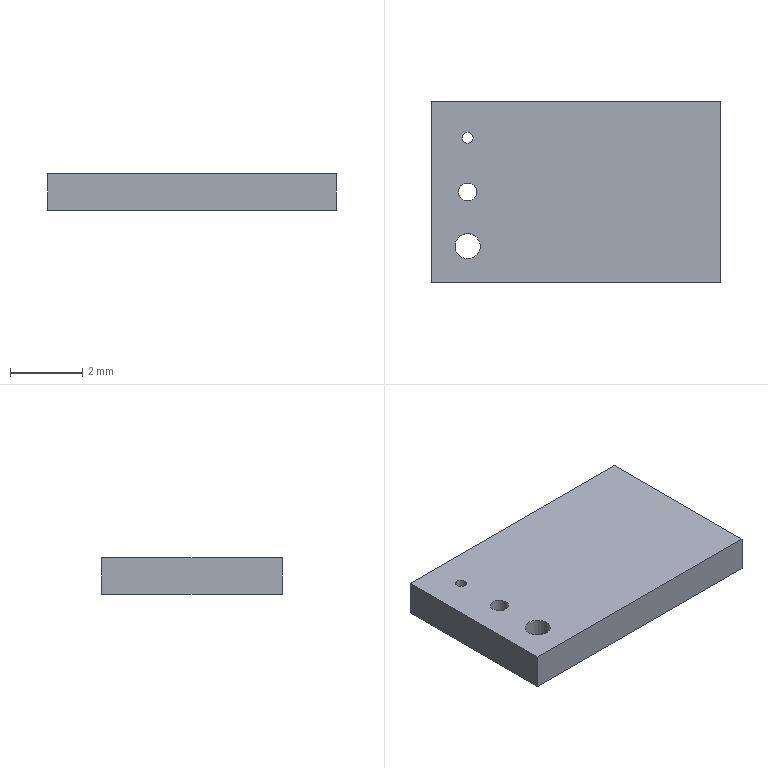Part | SolidWorks | features ICE 2, Extrusion 1 | 1 solid | 12 faces | box 8 x 5 x 1 mm | volume 39.348 mm3 | cylinder 6 | plane 6 | commonest cylinder face diameters 0.3 x2 0.5 x2 0.7 x2
STEP:
#1=CARTESIAN_POINT('',(0.85,-1.5,0.));
#2=VERTEX_POINT('',#1);
#3=CARTESIAN_POINT('',(1.15,-1.5,0.));
#4=VERTEX_POINT('',#3);
#5=CARTESIAN_POINT('',(1.,-1.5,0.));
#6=DIRECTION('',(0.,0.,1.));
#7=DIRECTION('',(1.,0.,0.));
#8=AXIS2_PLACEMENT_3D('',#5,#6,#7);
#9=CIRCLE('',#8,0.15);
#10=EDGE_CURVE('',#2,#4,#9,.T.);
#11=ORIENTED_EDGE('',*,*,#10,.F.);
#12=CARTESIAN_POINT('',(0.85,-1.5,1.));
#13=VERTEX_POINT('',#12);
#14=CARTESIAN_POINT('',(0.85,-1.5,-1.));
#15=DIRECTION('',(0.,0.,1.));
#16=VECTOR('',#15,1000.);
#17=LINE('',#14,#16);
#18=EDGE_CURVE('',#2,#13,#17,.T.);
#19=ORIENTED_EDGE('',*,*,#18,.T.);
#20=CARTESIAN_POINT('',(1.15,-1.5,1.));
#21=VERTEX_POINT('',#20);
#22=CARTESIAN_POINT('',(1.,-1.5,1.));
#23=DIRECTION('',(0.,0.,1.));
#24=DIRECTION('',(1.,0.,0.));
#25=AXIS2_PLACEMENT_3D('',#22,#23,#24);
#26=CIRCLE('',#25,0.15);
#27=EDGE_CURVE('',#13,#21,#26,.T.);
#28=ORIENTED_EDGE('',*,*,#27,.T.);
#29=CARTESIAN_POINT('',(1.15,-1.5,-1.));
#30=DIRECTION('',(0.,0.,1.));
#31=VECTOR('',#30,1000.);
#32=LINE('',#29,#31);
#33=EDGE_CURVE('',#4,#21,#32,.T.);
#34=ORIENTED_EDGE('',*,*,#33,.F.);
#35=EDGE_LOOP('',(#11,#19,#28,#34));
#36=FACE_OUTER_BOUND('',#35,.T.);
#37=CARTESIAN_POINT('',(1.,-1.5,-1.));
#38=DIRECTION('',(0.,0.,1.));
#39=DIRECTION('',(1.,0.,0.));
#40=AXIS2_PLACEMENT_3D('',#37,#38,#39);
#41=CYLINDRICAL_SURFACE('',#40,0.15);
#42=ADVANCED_FACE('',(#36),#41,.F.);
#43=CARTESIAN_POINT('',(0.75,-3.,0.));
#44=VERTEX_POINT('',#43);
#45=CARTESIAN_POINT('',(1.25,-3.,0.));
#46=VERTEX_POINT('',#45);
#47=CARTESIAN_POINT('',(1.,-3.,0.));
#48=DIRECTION('',(0.,0.,1.));
#49=DIRECTION('',(1.,0.,0.));
#50=AXIS2_PLACEMENT_3D('',#47,#48,#49);
#51=CIRCLE('',#50,0.25);
#52=EDGE_CURVE('',#44,#46,#51,.T.);
#53=ORIENTED_EDGE('',*,*,#52,.F.);
#54=CARTESIAN_POINT('',(0.75,-3.,1.));
#55=VERTEX_POINT('',#54);
#56=CARTESIAN_POINT('',(0.75,-3.,-1.));
#57=DIRECTION('',(0.,0.,1.));
#58=VECTOR('',#57,1000.);
#59=LINE('',#56,#58);
#60=EDGE_CURVE('',#44,#55,#59,.T.);
#61=ORIENTED_EDGE('',*,*,#60,.T.);
#62=CARTESIAN_POINT('',(1.25,-3.,1.));
#63=VERTEX_POINT('',#62);
#64=CARTESIAN_POINT('',(1.,-3.,1.));
#65=DIRECTION('',(0.,0.,1.));
#66=DIRECTION('',(1.,0.,0.));
#67=AXIS2_PLACEMENT_3D('',#64,#65,#66);
#68=CIRCLE('',#67,0.25);
#69=EDGE_CURVE('',#55,#63,#68,.T.);
#70=ORIENTED_EDGE('',*,*,#69,.T.);
#71=CARTESIAN_POINT('',(1.25,-3.,-1.));
#72=DIRECTION('',(0.,0.,1.));
#73=VECTOR('',#72,1000.);
#74=LINE('',#71,#73);
#75=EDGE_CURVE('',#46,#63,#74,.T.);
#76=ORIENTED_EDGE('',*,*,#75,.F.);
#77=EDGE_LOOP('',(#53,#61,#70,#76));
#78=FACE_OUTER_BOUND('',#77,.T.);
#79=CARTESIAN_POINT('',(1.,-3.,-1.));
#80=DIRECTION('',(0.,0.,1.));
#81=DIRECTION('',(1.,0.,0.));
#82=AXIS2_PLACEMENT_3D('',#79,#80,#81);
#83=CYLINDRICAL_SURFACE('',#82,0.25);
#84=ADVANCED_FACE('',(#78),#83,.F.);
#85=CARTESIAN_POINT('',(0.65,-4.5,0.));
#86=VERTEX_POINT('',#85);
#87=CARTESIAN_POINT('',(1.35,-4.5,0.));
#88=VERTEX_POINT('',#87);
#89=CARTESIAN_POINT('',(1.,-4.5,0.));
#90=DIRECTION('',(0.,0.,1.));
#91=DIRECTION('',(1.,0.,0.));
#92=AXIS2_PLACEMENT_3D('',#89,#90,#91);
#93=CIRCLE('',#92,0.35);
#94=EDGE_CURVE('',#86,#88,#93,.T.);
#95=ORIENTED_EDGE('',*,*,#94,.F.);
#96=CARTESIAN_POINT('',(0.65,-4.5,1.));
#97=VERTEX_POINT('',#96);
#98=CARTESIAN_POINT('',(0.65,-4.5,-1.));
#99=DIRECTION('',(0.,0.,1.));
#100=VECTOR('',#99,1000.);
#101=LINE('',#98,#100);
#102=EDGE_CURVE('',#86,#97,#101,.T.);
#103=ORIENTED_EDGE('',*,*,#102,.T.);
#104=CARTESIAN_POINT('',(1.35,-4.5,1.));
#105=VERTEX_POINT('',#104);
#106=CARTESIAN_POINT('',(1.,-4.5,1.));
#107=DIRECTION('',(0.,0.,1.));
#108=DIRECTION('',(1.,0.,0.));
#109=AXIS2_PLACEMENT_3D('',#106,#107,#108);
#110=CIRCLE('',#109,0.35);
#111=EDGE_CURVE('',#97,#105,#110,.T.);
#112=ORIENTED_EDGE('',*,*,#111,.T.);
#113=CARTESIAN_POINT('',(1.35,-4.5,-1.));
#114=DIRECTION('',(0.,0.,1.));
#115=VECTOR('',#114,1000.);
#116=LINE('',#113,#115);
#117=EDGE_CURVE('',#88,#105,#116,.T.);
#118=ORIENTED_EDGE('',*,*,#117,.F.);
#119=EDGE_LOOP('',(#95,#103,#112,#118));
#120=FACE_OUTER_BOUND('',#119,.T.);
#121=CARTESIAN_POINT('',(1.,-4.5,-1.));
#122=DIRECTION('',(0.,0.,1.));
#123=DIRECTION('',(1.,0.,0.));
#124=AXIS2_PLACEMENT_3D('',#121,#122,#123);
#125=CYLINDRICAL_SURFACE('',#124,0.35);
#126=ADVANCED_FACE('',(#120),#125,.F.);
#127=CARTESIAN_POINT('',(0.,-0.5,1.));
#128=VERTEX_POINT('',#127);
#129=CARTESIAN_POINT('',(0.,-5.5,1.));
#130=VERTEX_POINT('',#129);
#131=CARTESIAN_POINT('',(0.,0.,1.));
#132=DIRECTION('',(0.,-1.,0.));
#133=VECTOR('',#132,1000.);
#134=LINE('',#131,#133);
#135=EDGE_CURVE('',#128,#130,#134,.T.);
#136=ORIENTED_EDGE('',*,*,#135,.F.);
#137=CARTESIAN_POINT('',(0.,-0.5,0.));
#138=VERTEX_POINT('',#137);
#139=CARTESIAN_POINT('',(0.,-0.5,-6.));
#140=DIRECTION('',(0.,0.,1.));
#141=VECTOR('',#140,1000.);
#142=LINE('',#139,#141);
#143=EDGE_CURVE('',#138,#128,#142,.T.);
#144=ORIENTED_EDGE('',*,*,#143,.F.);
#145=CARTESIAN_POINT('',(0.,-5.5,0.));
#146=VERTEX_POINT('',#145);
#147=CARTESIAN_POINT('',(0.,0.,0.));
#148=DIRECTION('',(0.,-1.,0.));
#149=VECTOR('',#148,1000.);
#150=LINE('',#147,#149);
#151=EDGE_CURVE('',#138,#146,#150,.T.);
#152=ORIENTED_EDGE('',*,*,#151,.T.);
#153=CARTESIAN_POINT('',(0.,-5.5,-6.));
#154=DIRECTION('',(0.,0.,1.));
#155=VECTOR('',#154,1000.);
#156=LINE('',#153,#155);
#157=EDGE_CURVE('',#146,#130,#156,.T.);
#158=ORIENTED_EDGE('',*,*,#157,.T.);
#159=EDGE_LOOP('',(#136,#144,#152,#158));
#160=FACE_OUTER_BOUND('',#159,.T.);
#161=CARTESIAN_POINT('',(0.,0.,1.));
#162=DIRECTION('',(1.,0.,0.));
#163=DIRECTION('',(0.,1.,0.));
#164=AXIS2_PLACEMENT_3D('',#161,#162,#163);
#165=PLANE('',#164);
#166=ADVANCED_FACE('',(#160),#165,.F.);
#167=CARTESIAN_POINT('',(8.,-5.5,0.));
#168=VERTEX_POINT('',#167);
#169=CARTESIAN_POINT('',(8.,-0.5,0.));
#170=VERTEX_POINT('',#169);
#171=CARTESIAN_POINT('',(8.,0.,0.));
#172=DIRECTION('',(0.,1.,0.));
#173=VECTOR('',#172,1000.);
#174=LINE('',#171,#173);
#175=EDGE_CURVE('',#168,#170,#174,.T.);
#176=ORIENTED_EDGE('',*,*,#175,.T.);
#177=CARTESIAN_POINT('',(8.,-0.5,1.));
#178=VERTEX_POINT('',#177);
#179=CARTESIAN_POINT('',(8.,-0.5,-6.));
#180=DIRECTION('',(0.,0.,1.));
#181=VECTOR('',#180,1000.);
#182=LINE('',#179,#181);
#183=EDGE_CURVE('',#170,#178,#182,.T.);
#184=ORIENTED_EDGE('',*,*,#183,.T.);
#185=CARTESIAN_POINT('',(8.,-5.5,1.));
#186=VERTEX_POINT('',#185);
#187=CARTESIAN_POINT('',(8.,0.,1.));
#188=DIRECTION('',(0.,1.,0.));
#189=VECTOR('',#188,1000.);
#190=LINE('',#187,#189);
#191=EDGE_CURVE('',#186,#178,#190,.T.);
#192=ORIENTED_EDGE('',*,*,#191,.F.);
#193=CARTESIAN_POINT('',(8.,-5.5,-6.));
#194=DIRECTION('',(0.,0.,1.));
#195=VECTOR('',#194,1000.);
#196=LINE('',#193,#195);
#197=EDGE_CURVE('',#168,#186,#196,.T.);
#198=ORIENTED_EDGE('',*,*,#197,.F.);
#199=EDGE_LOOP('',(#176,#184,#192,#198));
#200=FACE_OUTER_BOUND('',#199,.T.);
#201=CARTESIAN_POINT('',(8.,0.,1.));
#202=DIRECTION('',(-1.,0.,0.));
#203=DIRECTION('',(0.,-1.,0.));
#204=AXIS2_PLACEMENT_3D('',#201,#202,#203);
#205=PLANE('',#204);
#206=ADVANCED_FACE('',(#200),#205,.F.);
#207=CARTESIAN_POINT('',(0.,-0.5,1.));
#208=DIRECTION('',(1.,0.,0.));
#209=VECTOR('',#208,1000.);
#210=LINE('',#207,#209);
#211=EDGE_CURVE('',#128,#178,#210,.T.);
#212=ORIENTED_EDGE('',*,*,#211,.F.);
#213=ORIENTED_EDGE('',*,*,#135,.T.);
#214=CARTESIAN_POINT('',(0.,-5.5,1.));
#215=DIRECTION('',(-1.,0.,0.));
#216=VECTOR('',#215,1000.);
#217=LINE('',#214,#216);
#218=EDGE_CURVE('',#186,#130,#217,.T.);
#219=ORIENTED_EDGE('',*,*,#218,.F.);
#220=ORIENTED_EDGE('',*,*,#191,.T.);
#221=EDGE_LOOP('',(#212,#213,#219,#220));
#222=FACE_OUTER_BOUND('',#221,.T.);
#223=CARTESIAN_POINT('',(1.,-1.5,1.));
#224=DIRECTION('',(0.,0.,1.));
#225=DIRECTION('',(1.,0.,0.));
#226=AXIS2_PLACEMENT_3D('',#223,#224,#225);
#227=CIRCLE('',#226,0.15);
#228=EDGE_CURVE('',#21,#13,#227,.T.);
#229=ORIENTED_EDGE('',*,*,#228,.F.);
#230=ORIENTED_EDGE('',*,*,#27,.F.);
#231=EDGE_LOOP('',(#229,#230));
#232=FACE_BOUND('',#231,.T.);
#233=CARTESIAN_POINT('',(1.,-3.,1.));
#234=DIRECTION('',(0.,0.,1.));
#235=DIRECTION('',(1.,0.,0.));
#236=AXIS2_PLACEMENT_3D('',#233,#234,#235);
#237=CIRCLE('',#236,0.25);
#238=EDGE_CURVE('',#63,#55,#237,.T.);
#239=ORIENTED_EDGE('',*,*,#238,.F.);
#240=ORIENTED_EDGE('',*,*,#69,.F.);
#241=EDGE_LOOP('',(#239,#240));
#242=FACE_BOUND('',#241,.T.);
#243=CARTESIAN_POINT('',(1.,-4.5,1.));
#244=DIRECTION('',(0.,0.,1.));
#245=DIRECTION('',(1.,0.,0.));
#246=AXIS2_PLACEMENT_3D('',#243,#244,#245);
#247=CIRCLE('',#246,0.35);
#248=EDGE_CURVE('',#105,#97,#247,.T.);
#249=ORIENTED_EDGE('',*,*,#248,.F.);
#250=ORIENTED_EDGE('',*,*,#111,.F.);
#251=EDGE_LOOP('',(#249,#250));
#252=FACE_BOUND('',#251,.T.);
#253=CARTESIAN_POINT('',(0.,0.,1.));
#254=DIRECTION('',(0.,0.,1.));
#255=DIRECTION('',(1.,0.,0.));
#256=AXIS2_PLACEMENT_3D('',#253,#254,#255);
#257=PLANE('',#256);
#258=ADVANCED_FACE('',(#222,#232,#242,#252),#257,.T.);
#259=CARTESIAN_POINT('',(1.,-1.5,0.));
#260=DIRECTION('',(0.,0.,1.));
#261=DIRECTION('',(1.,0.,0.));
#262=AXIS2_PLACEMENT_3D('',#259,#260,#261);
#263=CIRCLE('',#262,0.15);
#264=EDGE_CURVE('',#4,#2,#263,.T.);
#265=ORIENTED_EDGE('',*,*,#264,.T.);
#266=ORIENTED_EDGE('',*,*,#10,.T.);
#267=EDGE_LOOP('',(#265,#266));
#268=FACE_BOUND('',#267,.T.);
#269=CARTESIAN_POINT('',(1.,-3.,0.));
#270=DIRECTION('',(0.,0.,1.));
#271=DIRECTION('',(1.,0.,0.));
#272=AXIS2_PLACEMENT_3D('',#269,#270,#271);
#273=CIRCLE('',#272,0.25);
#274=EDGE_CURVE('',#46,#44,#273,.T.);
#275=ORIENTED_EDGE('',*,*,#274,.T.);
#276=ORIENTED_EDGE('',*,*,#52,.T.);
#277=EDGE_LOOP('',(#275,#276));
#278=FACE_BOUND('',#277,.T.);
#279=CARTESIAN_POINT('',(1.,-4.5,0.));
#280=DIRECTION('',(0.,0.,1.));
#281=DIRECTION('',(1.,0.,0.));
#282=AXIS2_PLACEMENT_3D('',#279,#280,#281);
#283=CIRCLE('',#282,0.35);
#284=EDGE_CURVE('',#88,#86,#283,.T.);
#285=ORIENTED_EDGE('',*,*,#284,.T.);
#286=ORIENTED_EDGE('',*,*,#94,.T.);
#287=EDGE_LOOP('',(#285,#286));
#288=FACE_BOUND('',#287,.T.);
#289=ORIENTED_EDGE('',*,*,#151,.F.);
#290=CARTESIAN_POINT('',(0.,-0.5,0.));
#291=DIRECTION('',(1.,0.,0.));
#292=VECTOR('',#291,1000.);
#293=LINE('',#290,#292);
#294=EDGE_CURVE('',#138,#170,#293,.T.);
#295=ORIENTED_EDGE('',*,*,#294,.T.);
#296=ORIENTED_EDGE('',*,*,#175,.F.);
#297=CARTESIAN_POINT('',(0.,-5.5,0.));
#298=DIRECTION('',(-1.,0.,0.));
#299=VECTOR('',#298,1000.);
#300=LINE('',#297,#299);
#301=EDGE_CURVE('',#168,#146,#300,.T.);
#302=ORIENTED_EDGE('',*,*,#301,.T.);
#303=EDGE_LOOP('',(#289,#295,#296,#302));
#304=FACE_OUTER_BOUND('',#303,.T.);
#305=CARTESIAN_POINT('',(0.,0.,0.));
#306=DIRECTION('',(0.,0.,1.));
#307=DIRECTION('',(1.,0.,0.));
#308=AXIS2_PLACEMENT_3D('',#305,#306,#307);
#309=PLANE('',#308);
#310=ADVANCED_FACE('',(#268,#278,#288,#304),#309,.F.);
#311=ORIENTED_EDGE('',*,*,#102,.F.);
#312=ORIENTED_EDGE('',*,*,#284,.F.);
#313=ORIENTED_EDGE('',*,*,#117,.T.);
#314=ORIENTED_EDGE('',*,*,#248,.T.);
#315=EDGE_LOOP('',(#311,#312,#313,#314));
#316=FACE_OUTER_BOUND('',#315,.T.);
#317=CARTESIAN_POINT('',(1.,-4.5,-1.));
#318=DIRECTION('',(0.,0.,1.));
#319=DIRECTION('',(1.,0.,0.));
#320=AXIS2_PLACEMENT_3D('',#317,#318,#319);
#321=CYLINDRICAL_SURFACE('',#320,0.35);
#322=ADVANCED_FACE('',(#316),#321,.F.);
#323=ORIENTED_EDGE('',*,*,#60,.F.);
#324=ORIENTED_EDGE('',*,*,#274,.F.);
#325=ORIENTED_EDGE('',*,*,#75,.T.);
#326=ORIENTED_EDGE('',*,*,#238,.T.);
#327=EDGE_LOOP('',(#323,#324,#325,#326));
#328=FACE_OUTER_BOUND('',#327,.T.);
#329=CARTESIAN_POINT('',(1.,-3.,-1.));
#330=DIRECTION('',(0.,0.,1.));
#331=DIRECTION('',(1.,0.,0.));
#332=AXIS2_PLACEMENT_3D('',#329,#330,#331);
#333=CYLINDRICAL_SURFACE('',#332,0.25);
#334=ADVANCED_FACE('',(#328),#333,.F.);
#335=ORIENTED_EDGE('',*,*,#18,.F.);
#336=ORIENTED_EDGE('',*,*,#264,.F.);
#337=ORIENTED_EDGE('',*,*,#33,.T.);
#338=ORIENTED_EDGE('',*,*,#228,.T.);
#339=EDGE_LOOP('',(#335,#336,#337,#338));
#340=FACE_OUTER_BOUND('',#339,.T.);
#341=CARTESIAN_POINT('',(1.,-1.5,-1.));
#342=DIRECTION('',(0.,0.,1.));
#343=DIRECTION('',(1.,0.,0.));
#344=AXIS2_PLACEMENT_3D('',#341,#342,#343);
#345=CYLINDRICAL_SURFACE('',#344,0.15);
#346=ADVANCED_FACE('',(#340),#345,.F.);
#347=ORIENTED_EDGE('',*,*,#197,.T.);
#348=ORIENTED_EDGE('',*,*,#218,.T.);
#349=ORIENTED_EDGE('',*,*,#157,.F.);
#350=ORIENTED_EDGE('',*,*,#301,.F.);
#351=EDGE_LOOP('',(#347,#348,#349,#350));
#352=FACE_OUTER_BOUND('',#351,.T.);
#353=CARTESIAN_POINT('',(0.,-5.5,-6.));
#354=DIRECTION('',(0.,1.,0.));
#355=DIRECTION('',(0.,0.,1.));
#356=AXIS2_PLACEMENT_3D('',#353,#354,#355);
#357=PLANE('',#356);
#358=ADVANCED_FACE('',(#352),#357,.F.);
#359=ORIENTED_EDGE('',*,*,#143,.T.);
#360=ORIENTED_EDGE('',*,*,#211,.T.);
#361=ORIENTED_EDGE('',*,*,#183,.F.);
#362=ORIENTED_EDGE('',*,*,#294,.F.);
#363=EDGE_LOOP('',(#359,#360,#361,#362));
#364=FACE_OUTER_BOUND('',#363,.T.);
#365=CARTESIAN_POINT('',(0.,-0.5,-6.));
#366=DIRECTION('',(0.,-1.,0.));
#367=DIRECTION('',(0.,0.,-1.));
#368=AXIS2_PLACEMENT_3D('',#365,#366,#367);
#369=PLANE('',#368);
#370=ADVANCED_FACE('',(#364),#369,.F.);
#371=CLOSED_SHELL('',(#42,#84,#126,#166,#206,#258,#310,#322,#334,#346,#358,#370));
#372=MANIFOLD_SOLID_BREP('',#371);
#373=CARTESIAN_POINT('',(0.,0.,0.));
#374=DIRECTION('',(0.,0.,1.));
#375=DIRECTION('',(1.,0.,0.));
#376=AXIS2_PLACEMENT_3D('',#373,#374,#375);
#377=(LENGTH_UNIT()NAMED_UNIT(*)SI_UNIT(.MILLI.,.METRE.));
#378=UNCERTAINTY_MEASURE_WITH_UNIT(LENGTH_MEASURE(0.00001),#377,'','');
#379=(NAMED_UNIT(*)PLANE_ANGLE_UNIT()SI_UNIT($,.RADIAN.));
#380=(NAMED_UNIT(*)SI_UNIT($,.STERADIAN.)SOLID_ANGLE_UNIT());
#381=(GEOMETRIC_REPRESENTATION_CONTEXT(3)GLOBAL_UNCERTAINTY_ASSIGNED_CONTEXT((#378))GLOBAL_UNIT_ASSIGNED_CONTEXT((#377,#379,#380))REPRESENTATION_CONTEXT('',''));
#382=ADVANCED_BREP_SHAPE_REPRESENTATION('',(#372,#376),#381);